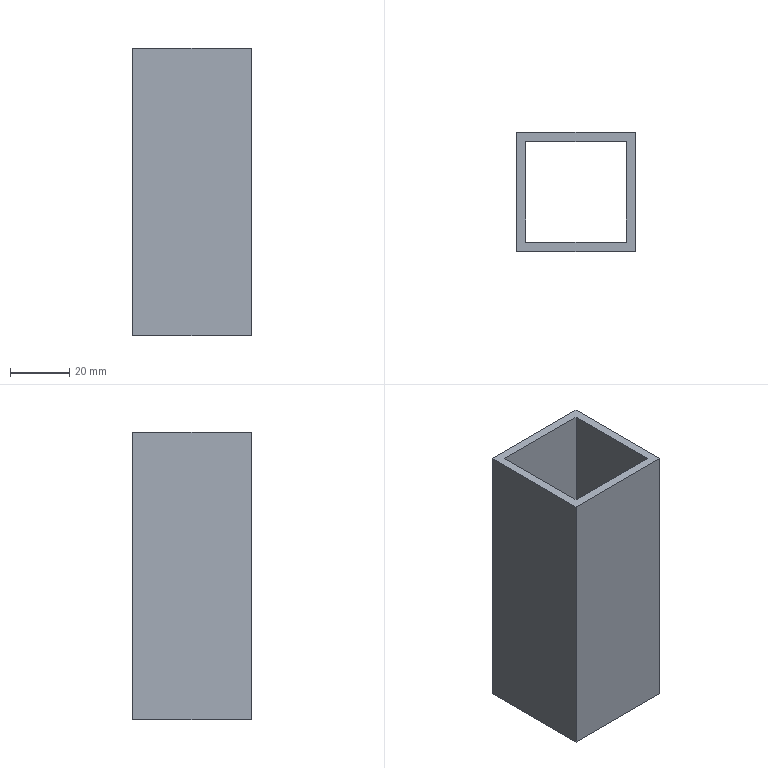Part | SolidWorks | features Extrusion 1 | 1 solid | 10 faces | box 40 x 40 x 97 mm | volume 43068 mm3 | plane 10
STEP:
#1=CARTESIAN_POINT('',(-20.,20.,48.5));
#2=VERTEX_POINT('',#1);
#3=CARTESIAN_POINT('',(-20.,-20.,48.5));
#4=VERTEX_POINT('',#3);
#5=CARTESIAN_POINT('',(-20.,20.,48.5));
#6=DIRECTION('',(0.,-1.,0.));
#7=VECTOR('',#6,1000.);
#8=LINE('',#5,#7);
#9=EDGE_CURVE('',#2,#4,#8,.T.);
#10=ORIENTED_EDGE('',*,*,#9,.F.);
#11=CARTESIAN_POINT('',(-20.,20.,-48.5));
#12=VERTEX_POINT('',#11);
#13=CARTESIAN_POINT('',(-20.,20.,-48.5));
#14=DIRECTION('',(0.,0.,1.));
#15=VECTOR('',#14,1000.);
#16=LINE('',#13,#15);
#17=EDGE_CURVE('',#12,#2,#16,.T.);
#18=ORIENTED_EDGE('',*,*,#17,.F.);
#19=CARTESIAN_POINT('',(-20.,-20.,-48.5));
#20=VERTEX_POINT('',#19);
#21=CARTESIAN_POINT('',(-20.,20.,-48.5));
#22=DIRECTION('',(0.,-1.,0.));
#23=VECTOR('',#22,1000.);
#24=LINE('',#21,#23);
#25=EDGE_CURVE('',#12,#20,#24,.T.);
#26=ORIENTED_EDGE('',*,*,#25,.T.);
#27=CARTESIAN_POINT('',(-20.,-20.,-48.5));
#28=DIRECTION('',(0.,0.,1.));
#29=VECTOR('',#28,1000.);
#30=LINE('',#27,#29);
#31=EDGE_CURVE('',#20,#4,#30,.T.);
#32=ORIENTED_EDGE('',*,*,#31,.T.);
#33=EDGE_LOOP('',(#10,#18,#26,#32));
#34=FACE_OUTER_BOUND('',#33,.T.);
#35=CARTESIAN_POINT('',(-20.,20.,-48.5));
#36=DIRECTION('',(-1.,0.,0.));
#37=DIRECTION('',(0.,0.,1.));
#38=AXIS2_PLACEMENT_3D('',#35,#36,#37);
#39=PLANE('',#38);
#40=ADVANCED_FACE('',(#34),#39,.T.);
#41=CARTESIAN_POINT('',(20.,20.,48.5));
#42=VERTEX_POINT('',#41);
#43=CARTESIAN_POINT('',(20.,20.,48.5));
#44=DIRECTION('',(-1.,0.,0.));
#45=VECTOR('',#44,1000.);
#46=LINE('',#43,#45);
#47=EDGE_CURVE('',#42,#2,#46,.T.);
#48=ORIENTED_EDGE('',*,*,#47,.F.);
#49=CARTESIAN_POINT('',(20.,20.,-48.5));
#50=VERTEX_POINT('',#49);
#51=CARTESIAN_POINT('',(20.,20.,-48.5));
#52=DIRECTION('',(0.,0.,1.));
#53=VECTOR('',#52,1000.);
#54=LINE('',#51,#53);
#55=EDGE_CURVE('',#50,#42,#54,.T.);
#56=ORIENTED_EDGE('',*,*,#55,.F.);
#57=CARTESIAN_POINT('',(20.,20.,-48.5));
#58=DIRECTION('',(-1.,0.,0.));
#59=VECTOR('',#58,1000.);
#60=LINE('',#57,#59);
#61=EDGE_CURVE('',#50,#12,#60,.T.);
#62=ORIENTED_EDGE('',*,*,#61,.T.);
#63=ORIENTED_EDGE('',*,*,#17,.T.);
#64=EDGE_LOOP('',(#48,#56,#62,#63));
#65=FACE_OUTER_BOUND('',#64,.T.);
#66=CARTESIAN_POINT('',(20.,20.,-48.5));
#67=DIRECTION('',(0.,1.,0.));
#68=DIRECTION('',(0.,0.,1.));
#69=AXIS2_PLACEMENT_3D('',#66,#67,#68);
#70=PLANE('',#69);
#71=ADVANCED_FACE('',(#65),#70,.T.);
#72=CARTESIAN_POINT('',(20.,-20.,48.5));
#73=VERTEX_POINT('',#72);
#74=CARTESIAN_POINT('',(20.,-20.,48.5));
#75=DIRECTION('',(0.,1.,0.));
#76=VECTOR('',#75,1000.);
#77=LINE('',#74,#76);
#78=EDGE_CURVE('',#73,#42,#77,.T.);
#79=ORIENTED_EDGE('',*,*,#78,.F.);
#80=CARTESIAN_POINT('',(20.,-20.,-48.5));
#81=VERTEX_POINT('',#80);
#82=CARTESIAN_POINT('',(20.,-20.,-48.5));
#83=DIRECTION('',(0.,0.,1.));
#84=VECTOR('',#83,1000.);
#85=LINE('',#82,#84);
#86=EDGE_CURVE('',#81,#73,#85,.T.);
#87=ORIENTED_EDGE('',*,*,#86,.F.);
#88=CARTESIAN_POINT('',(20.,-20.,-48.5));
#89=DIRECTION('',(0.,1.,0.));
#90=VECTOR('',#89,1000.);
#91=LINE('',#88,#90);
#92=EDGE_CURVE('',#81,#50,#91,.T.);
#93=ORIENTED_EDGE('',*,*,#92,.T.);
#94=ORIENTED_EDGE('',*,*,#55,.T.);
#95=EDGE_LOOP('',(#79,#87,#93,#94));
#96=FACE_OUTER_BOUND('',#95,.T.);
#97=CARTESIAN_POINT('',(20.,-20.,-48.5));
#98=DIRECTION('',(1.,0.,0.));
#99=DIRECTION('',(0.,0.,-1.));
#100=AXIS2_PLACEMENT_3D('',#97,#98,#99);
#101=PLANE('',#100);
#102=ADVANCED_FACE('',(#96),#101,.T.);
#103=CARTESIAN_POINT('',(-20.,-20.,48.5));
#104=DIRECTION('',(1.,0.,0.));
#105=VECTOR('',#104,1000.);
#106=LINE('',#103,#105);
#107=EDGE_CURVE('',#4,#73,#106,.T.);
#108=ORIENTED_EDGE('',*,*,#107,.F.);
#109=ORIENTED_EDGE('',*,*,#31,.F.);
#110=CARTESIAN_POINT('',(-20.,-20.,-48.5));
#111=DIRECTION('',(1.,0.,0.));
#112=VECTOR('',#111,1000.);
#113=LINE('',#110,#112);
#114=EDGE_CURVE('',#20,#81,#113,.T.);
#115=ORIENTED_EDGE('',*,*,#114,.T.);
#116=ORIENTED_EDGE('',*,*,#86,.T.);
#117=EDGE_LOOP('',(#108,#109,#115,#116));
#118=FACE_OUTER_BOUND('',#117,.T.);
#119=CARTESIAN_POINT('',(-20.,-20.,-48.5));
#120=DIRECTION('',(0.,-1.,0.));
#121=DIRECTION('',(0.,0.,-1.));
#122=AXIS2_PLACEMENT_3D('',#119,#120,#121);
#123=PLANE('',#122);
#124=ADVANCED_FACE('',(#118),#123,.T.);
#125=CARTESIAN_POINT('',(17.,17.,-48.5));
#126=VERTEX_POINT('',#125);
#127=CARTESIAN_POINT('',(-17.,17.,-48.5));
#128=VERTEX_POINT('',#127);
#129=CARTESIAN_POINT('',(17.,17.,-48.5));
#130=DIRECTION('',(-1.,0.,0.));
#131=VECTOR('',#130,1000.);
#132=LINE('',#129,#131);
#133=EDGE_CURVE('',#126,#128,#132,.T.);
#134=ORIENTED_EDGE('',*,*,#133,.T.);
#135=CARTESIAN_POINT('',(-17.,-17.,-48.5));
#136=VERTEX_POINT('',#135);
#137=CARTESIAN_POINT('',(-17.,17.,-48.5));
#138=DIRECTION('',(0.,-1.,0.));
#139=VECTOR('',#138,1000.);
#140=LINE('',#137,#139);
#141=EDGE_CURVE('',#128,#136,#140,.T.);
#142=ORIENTED_EDGE('',*,*,#141,.T.);
#143=CARTESIAN_POINT('',(17.,-17.,-48.5));
#144=VERTEX_POINT('',#143);
#145=CARTESIAN_POINT('',(-17.,-17.,-48.5));
#146=DIRECTION('',(1.,0.,0.));
#147=VECTOR('',#146,1000.);
#148=LINE('',#145,#147);
#149=EDGE_CURVE('',#136,#144,#148,.T.);
#150=ORIENTED_EDGE('',*,*,#149,.T.);
#151=CARTESIAN_POINT('',(17.,-17.,-48.5));
#152=DIRECTION('',(0.,1.,0.));
#153=VECTOR('',#152,1000.);
#154=LINE('',#151,#153);
#155=EDGE_CURVE('',#144,#126,#154,.T.);
#156=ORIENTED_EDGE('',*,*,#155,.T.);
#157=EDGE_LOOP('',(#134,#142,#150,#156));
#158=FACE_BOUND('',#157,.T.);
#159=ORIENTED_EDGE('',*,*,#25,.F.);
#160=ORIENTED_EDGE('',*,*,#61,.F.);
#161=ORIENTED_EDGE('',*,*,#92,.F.);
#162=ORIENTED_EDGE('',*,*,#114,.F.);
#163=EDGE_LOOP('',(#159,#160,#161,#162));
#164=FACE_OUTER_BOUND('',#163,.T.);
#165=CARTESIAN_POINT('',(0.,0.,-48.5));
#166=DIRECTION('',(0.,0.,1.));
#167=DIRECTION('',(1.,0.,0.));
#168=AXIS2_PLACEMENT_3D('',#165,#166,#167);
#169=PLANE('',#168);
#170=ADVANCED_FACE('',(#158,#164),#169,.F.);
#171=CARTESIAN_POINT('',(-17.,17.,48.5));
#172=VERTEX_POINT('',#171);
#173=CARTESIAN_POINT('',(-17.,-17.,48.5));
#174=VERTEX_POINT('',#173);
#175=CARTESIAN_POINT('',(-17.,17.,48.5));
#176=DIRECTION('',(0.,-1.,0.));
#177=VECTOR('',#176,1000.);
#178=LINE('',#175,#177);
#179=EDGE_CURVE('',#172,#174,#178,.T.);
#180=ORIENTED_EDGE('',*,*,#179,.F.);
#181=CARTESIAN_POINT('',(17.,17.,48.5));
#182=VERTEX_POINT('',#181);
#183=CARTESIAN_POINT('',(17.,17.,48.5));
#184=DIRECTION('',(-1.,0.,0.));
#185=VECTOR('',#184,1000.);
#186=LINE('',#183,#185);
#187=EDGE_CURVE('',#182,#172,#186,.T.);
#188=ORIENTED_EDGE('',*,*,#187,.F.);
#189=CARTESIAN_POINT('',(17.,-17.,48.5));
#190=VERTEX_POINT('',#189);
#191=CARTESIAN_POINT('',(17.,-17.,48.5));
#192=DIRECTION('',(0.,1.,0.));
#193=VECTOR('',#192,1000.);
#194=LINE('',#191,#193);
#195=EDGE_CURVE('',#190,#182,#194,.T.);
#196=ORIENTED_EDGE('',*,*,#195,.F.);
#197=CARTESIAN_POINT('',(-17.,-17.,48.5));
#198=DIRECTION('',(1.,0.,0.));
#199=VECTOR('',#198,1000.);
#200=LINE('',#197,#199);
#201=EDGE_CURVE('',#174,#190,#200,.T.);
#202=ORIENTED_EDGE('',*,*,#201,.F.);
#203=EDGE_LOOP('',(#180,#188,#196,#202));
#204=FACE_BOUND('',#203,.T.);
#205=ORIENTED_EDGE('',*,*,#9,.T.);
#206=ORIENTED_EDGE('',*,*,#107,.T.);
#207=ORIENTED_EDGE('',*,*,#78,.T.);
#208=ORIENTED_EDGE('',*,*,#47,.T.);
#209=EDGE_LOOP('',(#205,#206,#207,#208));
#210=FACE_OUTER_BOUND('',#209,.T.);
#211=CARTESIAN_POINT('',(0.,0.,48.5));
#212=DIRECTION('',(0.,0.,1.));
#213=DIRECTION('',(1.,0.,0.));
#214=AXIS2_PLACEMENT_3D('',#211,#212,#213);
#215=PLANE('',#214);
#216=ADVANCED_FACE('',(#204,#210),#215,.T.);
#217=ORIENTED_EDGE('',*,*,#179,.T.);
#218=CARTESIAN_POINT('',(-17.,-17.,-48.5));
#219=DIRECTION('',(0.,0.,1.));
#220=VECTOR('',#219,1000.);
#221=LINE('',#218,#220);
#222=EDGE_CURVE('',#136,#174,#221,.T.);
#223=ORIENTED_EDGE('',*,*,#222,.F.);
#224=ORIENTED_EDGE('',*,*,#141,.F.);
#225=CARTESIAN_POINT('',(-17.,17.,-48.5));
#226=DIRECTION('',(0.,0.,1.));
#227=VECTOR('',#226,1000.);
#228=LINE('',#225,#227);
#229=EDGE_CURVE('',#128,#172,#228,.T.);
#230=ORIENTED_EDGE('',*,*,#229,.T.);
#231=EDGE_LOOP('',(#217,#223,#224,#230));
#232=FACE_OUTER_BOUND('',#231,.T.);
#233=CARTESIAN_POINT('',(-17.,17.,-48.5));
#234=DIRECTION('',(-1.,0.,0.));
#235=DIRECTION('',(0.,0.,1.));
#236=AXIS2_PLACEMENT_3D('',#233,#234,#235);
#237=PLANE('',#236);
#238=ADVANCED_FACE('',(#232),#237,.F.);
#239=ORIENTED_EDGE('',*,*,#187,.T.);
#240=ORIENTED_EDGE('',*,*,#229,.F.);
#241=ORIENTED_EDGE('',*,*,#133,.F.);
#242=CARTESIAN_POINT('',(17.,17.,-48.5));
#243=DIRECTION('',(0.,0.,1.));
#244=VECTOR('',#243,1000.);
#245=LINE('',#242,#244);
#246=EDGE_CURVE('',#126,#182,#245,.T.);
#247=ORIENTED_EDGE('',*,*,#246,.T.);
#248=EDGE_LOOP('',(#239,#240,#241,#247));
#249=FACE_OUTER_BOUND('',#248,.T.);
#250=CARTESIAN_POINT('',(17.,17.,-48.5));
#251=DIRECTION('',(0.,1.,0.));
#252=DIRECTION('',(0.,0.,1.));
#253=AXIS2_PLACEMENT_3D('',#250,#251,#252);
#254=PLANE('',#253);
#255=ADVANCED_FACE('',(#249),#254,.F.);
#256=ORIENTED_EDGE('',*,*,#195,.T.);
#257=ORIENTED_EDGE('',*,*,#246,.F.);
#258=ORIENTED_EDGE('',*,*,#155,.F.);
#259=CARTESIAN_POINT('',(17.,-17.,-48.5));
#260=DIRECTION('',(0.,0.,1.));
#261=VECTOR('',#260,1000.);
#262=LINE('',#259,#261);
#263=EDGE_CURVE('',#144,#190,#262,.T.);
#264=ORIENTED_EDGE('',*,*,#263,.T.);
#265=EDGE_LOOP('',(#256,#257,#258,#264));
#266=FACE_OUTER_BOUND('',#265,.T.);
#267=CARTESIAN_POINT('',(17.,-17.,-48.5));
#268=DIRECTION('',(1.,0.,0.));
#269=DIRECTION('',(0.,0.,-1.));
#270=AXIS2_PLACEMENT_3D('',#267,#268,#269);
#271=PLANE('',#270);
#272=ADVANCED_FACE('',(#266),#271,.F.);
#273=ORIENTED_EDGE('',*,*,#201,.T.);
#274=ORIENTED_EDGE('',*,*,#263,.F.);
#275=ORIENTED_EDGE('',*,*,#149,.F.);
#276=ORIENTED_EDGE('',*,*,#222,.T.);
#277=EDGE_LOOP('',(#273,#274,#275,#276));
#278=FACE_OUTER_BOUND('',#277,.T.);
#279=CARTESIAN_POINT('',(-17.,-17.,-48.5));
#280=DIRECTION('',(0.,-1.,0.));
#281=DIRECTION('',(0.,0.,-1.));
#282=AXIS2_PLACEMENT_3D('',#279,#280,#281);
#283=PLANE('',#282);
#284=ADVANCED_FACE('',(#278),#283,.F.);
#285=CLOSED_SHELL('',(#40,#71,#102,#124,#170,#216,#238,#255,#272,#284));
#286=MANIFOLD_SOLID_BREP('',#285);
#287=CARTESIAN_POINT('',(0.,0.,0.));
#288=DIRECTION('',(0.,0.,1.));
#289=DIRECTION('',(1.,0.,0.));
#290=AXIS2_PLACEMENT_3D('',#287,#288,#289);
#291=(LENGTH_UNIT()NAMED_UNIT(*)SI_UNIT(.MILLI.,.METRE.));
#292=UNCERTAINTY_MEASURE_WITH_UNIT(LENGTH_MEASURE(0.00001),#291,'','');
#293=(NAMED_UNIT(*)PLANE_ANGLE_UNIT()SI_UNIT($,.RADIAN.));
#294=(NAMED_UNIT(*)SI_UNIT($,.STERADIAN.)SOLID_ANGLE_UNIT());
#295=(GEOMETRIC_REPRESENTATION_CONTEXT(3)GLOBAL_UNCERTAINTY_ASSIGNED_CONTEXT((#292))GLOBAL_UNIT_ASSIGNED_CONTEXT((#291,#293,#294))REPRESENTATION_CONTEXT('',''));
#296=ADVANCED_BREP_SHAPE_REPRESENTATION('',(#286,#290),#295);